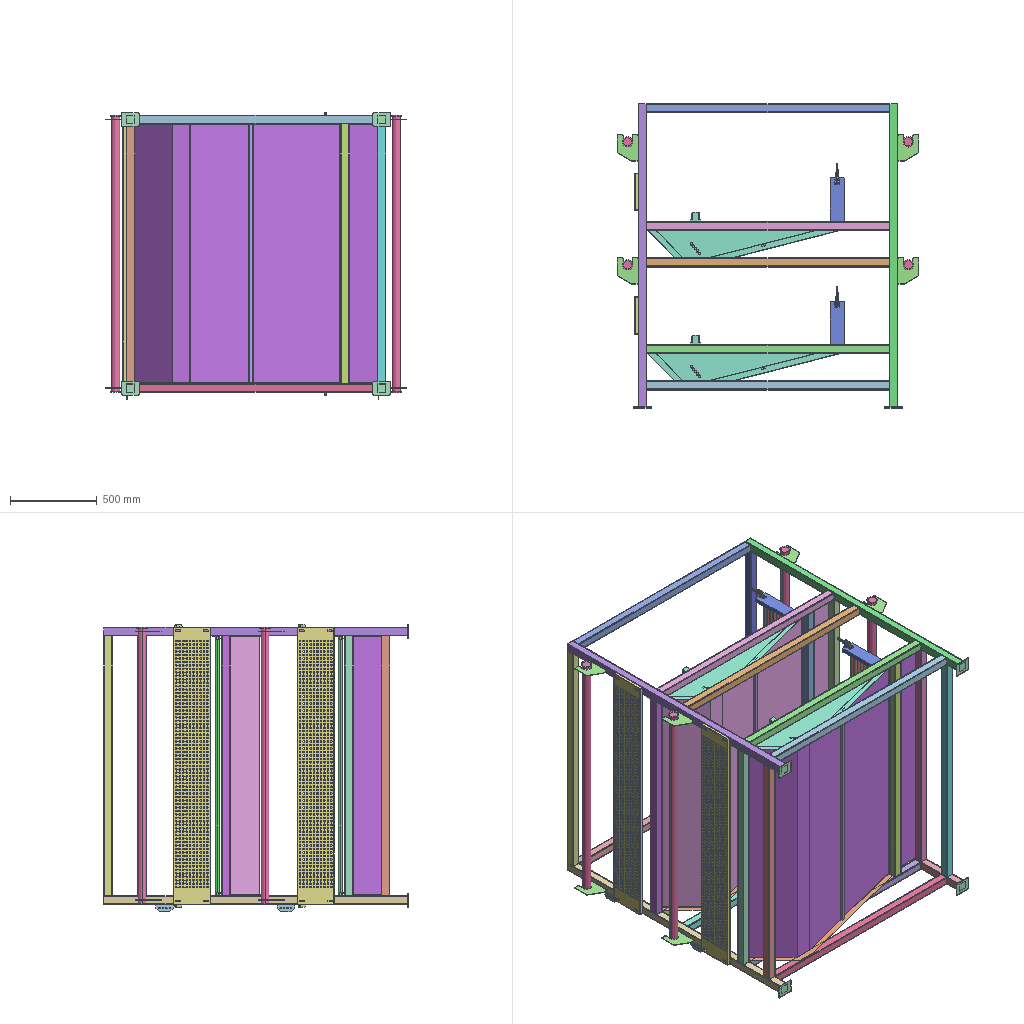Assembly | SolidWorks | 29 different items | 101 placed | box 1740 x 1755 x 1658 mm
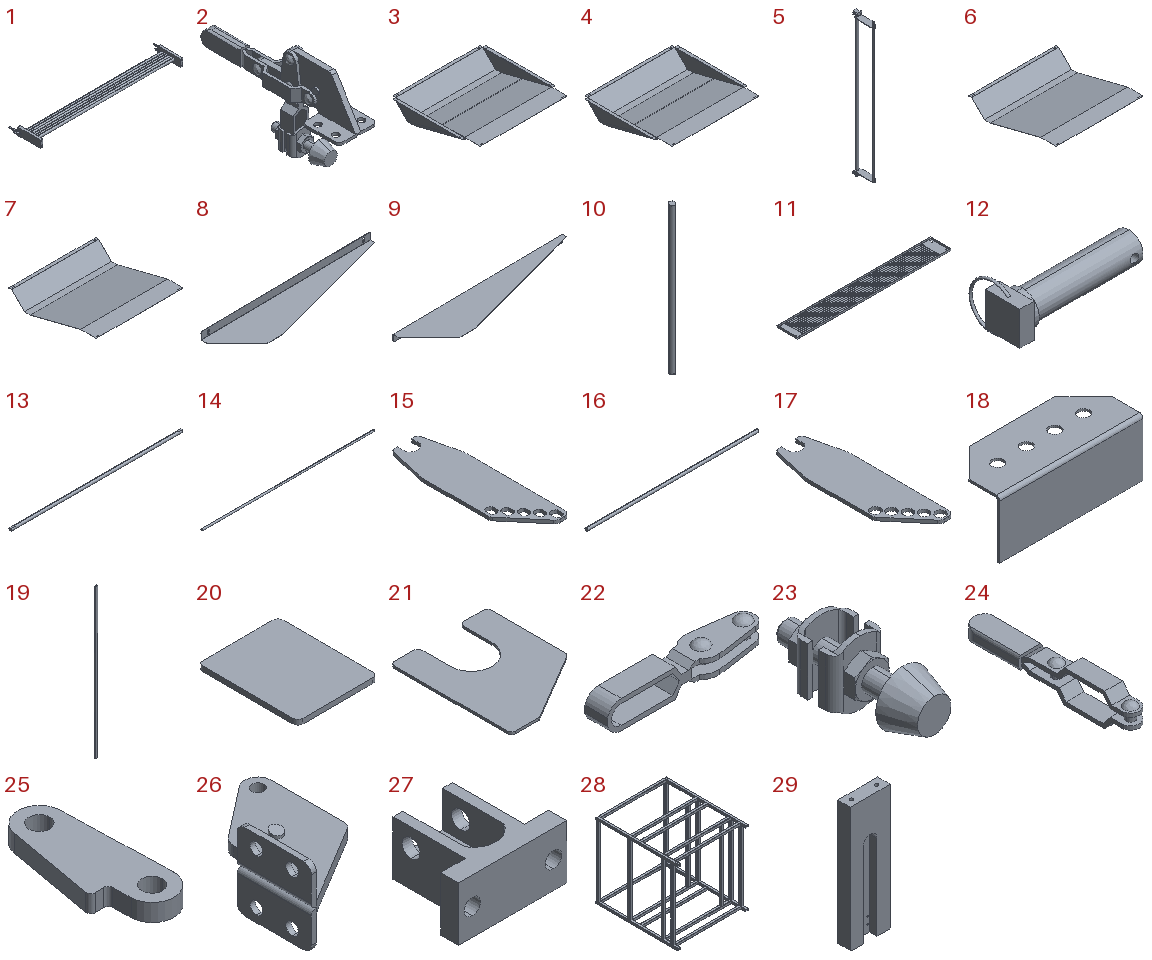Parts list (item | name | quantity | parent item | size | volume | features):
1 | (subassembly) | x2 | - | 1633 x 333.3 x 80 mm | 5408151 mm3 | features ReferencePattern 5, AEMSimFeature 1, LocalLPattern 1
2 | (subassembly) | x4 | in 1 | 30 x 119.8 x 70.25 mm | 20145 mm3 | -
3 | (subassembly) | x1 | - | 1590 x 1497 x 254.534 mm | 4476617 mm3 | -
4 | (subassembly) | x1 | - | 1590 x 1497 x 255.323 mm | 4476617 mm3 | -
5 | (subassembly) | x2 | - | 68 x 247.07 x 1556 mm | 2258393 mm3 | features ReferencePattern 4, LocalLPattern 1
6 | - | x1 | in 3 | 1490 x 1497 x 221.028 mm | 3607378 mm3 | features EdgeFlange 4, Extrusion 1, Fillet 1, FlatPattern 1, ICE 1, SheetMetal 1, SolidToSheetMetal 1
7 | - | x1 | in 4 | 1490 x 1497 x 221.028 mm | 3607378 mm3 | features EdgeFlange 4, Extrusion 1, Fillet 1, FlatPattern 1, ICE 1, SheetMetal 1, SolidToSheetMetal 1
8 | - | x2 | in 3, 4 | 1189 x 264.437 x 50 mm | 360864 mm3 | features EdgeFlange 1, Extrusion 1, Fillet 1, FlatPattern 1, ICE 1, SheetMetal 1, SolidToSheetMetal 1
9 | - | x2 | in 3, 4 | 1189 x 264.437 x 50 mm | 360864 mm3 | features EdgeFlange 1, Extrusion 1, Fillet 1, FlatPattern 1, ICE 1, SheetMetal 1, SolidToSheetMetal 1
10 | - | x4 | - | 60 x 60 x 1600 mm | 273036 mm3 | features ICE 2, Extrusion 1, Fillet 1, RefAxis 1, RevCut 1
11 | - | x2 | - | 1600 x 215 x 20 mm | 538674 mm3 | features ICE 3, EdgeFlange 1, Extrusion 1, FlatPattern 1, SheetMetal 1, SolidToSheetMetal 1
12 | - | x4 | in 5 | 45 x 19.844 x 16.686 mm | 3901 mm3 | features ICE 3, BaseBody 1, Sweep 1
13 | - | x2 | in 5 | 1530 x 25 x 25 mm | 749305 mm3 | features ICE 3, Extrusion 1, HoleWzd 1
14 | - | x10 | in 5 | 1480 x 15 x 15 mm | 261335 mm3 | features HoleWzd 2, Chamfer 1, Extrusion 1, ICE 1
15 | - | x2 | in 5 | 68 x 225 x 5 mm | 59113 mm3 | features Fillet 5, ICE 5, Extrusion 1, LPattern 1
16 | - | x12 | in 1 | 1534 x 25 x 25 mm | 753000 mm3 | features ICE 1, MirrorPattern 1, Revolution 1
17 | - | x2 | in 5 | 68 x 225 x 5 mm | 58604 mm3 | features Fillet 5, ICE 4, Extrusion 1
18 | - | x4 | - | 100 x 41.5 x 40 mm | 10986 mm3 | features Chamfer 1, EdgeFlange 1, Extrusion 1, FlatPattern 1, SheetMetal 1, SolidToSheetMetal 1
19 | - | x2 | in 3, 4 | 23 x 13 x 1490 mm | 147510 mm3 | features ExtruThin 1, WeldmentFeature 1
20 | - | x4 | - | 80 x 100 x 5 mm | 39893 mm3 | features Extrusion 1, Fillet 1
21 | - | x8 | - | 120 x 150 x 3 mm | 38115 mm3 | features Extrusion 1
22 | - | x4 | in 2 | 70.05 x 15.001 x 12.4 mm | 3515 mm3 | features BaseBody 1
23 | - | x4 | in 2 | 16 x 44.45 x 19 mm | 3867 mm3 | features BaseBody 1
24 | - | x4 | in 2 | 12.6 x 89.5 x 17.6 mm | 5262 mm3 | features BaseBody 1
25 | - | x4 | in 2 | 14.127 x 35.318 x 4 mm | 1354 mm3 | features BaseBody 1
26 | - | x4 | in 2 | 34.2 x 55.001 x 30 mm | 6148 mm3 | features BaseBody 1
27 | - | x4 | in 5 | 60 x 50 x 30 mm | 38448 mm3 | features HoleWzd 3, ICE 3, Extrusion 1
28 | - | x1 | - | 1500 x 1750 x 1600 mm | 13453168 mm3 | features 3DProfileFeature 1, WeldCornerFeat 1, WeldMemberFeat 1, WeldmentFeature 1
29 | - | x4 | in 1 | 80 x 25 x 250 mm | 424930 mm3 | features HoleWzd 5, ICE 2, MirrorPattern 2, Chamfer 1, Extrusion 1
Mates (type | each side: item.copy, entity, surface, feature):
In the top assembly
Coincident | 28.1 face plane GB 6728-1986 square hollow section 050 X 50 X 2 | 6.1 face plane Convert entities1 | 2 times
Width | 28.1 face plane GB 6728-1986 square hollow section 050 X 50 X 2 | 28.1 face plane GB 6728-1986 square hollow section 050 X 50 X 2 | 9.1 face plane Convert entities1 | 8.1 face plane Convert entities1
Coincident | 28.1 face plane GB 6728-1986 square hollow section 050 X 50 X 2 | 21.1 face plane Boss-Extrude1
Coincident | 28.1 face plane GB 6728-1986 square hollow section 050 X 50 X 2 | 21.2 face plane Boss-Extrude1
Coincident | 28.1 face plane GB 6728-1986 square hollow section 050 X 50 X 2 | 21.3 face plane Boss-Extrude1
Coincident | 28.1 face plane GB 6728-1986 square hollow section 050 X 50 X 2 | 21.4 face plane Boss-Extrude1
Width | 28.1 face plane GB 6728-1986 square hollow section 050 X 50 X 2 | 28.1 face plane GB 6728-1986 square hollow section 050 X 50 X 2 | 21.3 face plane Boss-Extrude1 | 21.3 face plane Boss-Extrude1
Width | 28.1 face plane GB 6728-1986 square hollow section 050 X 50 X 2 | 28.1 face plane GB 6728-1986 square hollow section 050 X 50 X 2 | 21.1 face plane Boss-Extrude1 | 21.1 face plane Boss-Extrude1
Coincident | 21.3 face plane Boss-Extrude1 | 21.1 face plane Boss-Extrude1
Coincident | 21.1 face plane Boss-Extrude1 | 21.2 face plane Boss-Extrude1
Coincident | 21.2 face plane Boss-Extrude1 | 21.4 face plane Boss-Extrude1
Width | 28.1 face plane GB 6728-1986 square hollow section 050 X 50 X 2 | 28.1 face plane GB 6728-1986 square hollow section 050 X 50 X 2 | 21.2 face plane Boss-Extrude1 | 21.2 face plane Boss-Extrude1
Width | 28.1 face plane GB 6728-1986 square hollow section 050 X 50 X 2 | 28.1 face plane GB 6728-1986 square hollow section 050 X 50 X 2 | 21.4 face plane Boss-Extrude1 | 21.4 face plane Boss-Extrude1
DistanceDim | 28.1 face plane GB 6728-1986 square hollow section 050 X 50 X 2 | 21.4 face plane Boss-Extrude1
Coincident | 21.4 face plane Boss-Extrude1 | 21.5 face plane Boss-Extrude1
Coincident | 28.1 face plane GB 6728-1986 square hollow section 050 X 50 X 2 | 21.5 face plane Boss-Extrude1
Coincident | 21.1 face plane Boss-Extrude1 | 21.6 face plane Boss-Extrude1
Coincident | 28.1 face plane GB 6728-1986 square hollow section 050 X 50 X 2 | 21.6 face plane Boss-Extrude1
Coincident | 21.3 face plane Boss-Extrude1 | 21.7 face plane Boss-Extrude1
Coincident | 28.1 face plane GB 6728-1986 square hollow section 050 X 50 X 2 | 21.7 face plane Boss-Extrude1
Coincident | 28.1 face plane GB 6728-1986 square hollow section 050 X 50 X 2 | 21.8 face plane Boss-Extrude1
Coincident | 21.2 face plane Boss-Extrude1 | 21.8 face plane Boss-Extrude1
Coincident | 21.5 face plane Boss-Extrude1 | 21.8 face plane Boss-Extrude1
Coincident | 21.7 face plane Boss-Extrude1 | 21.6 face plane Boss-Extrude1
Coincident | 21.7 face plane Boss-Extrude1 | 21.8 face plane Boss-Extrude1
Concentric | 21.3 edge | 10.1 face cylinder Boss-Extrude1
Width | 28.1 face plane GB 6728-1986 square hollow section 050 X 50 X 2 | 28.1 face plane GB 6728-1986 square hollow section 050 X 50 X 2 | 10.1 face plane Boss-Extrude3 | 10.1 face plane Boss-Extrude2
Concentric | 21.7 edge | 10.2 face cylinder Boss-Extrude1
Concentric | 21.2 edge | 10.3 face cylinder Boss-Extrude1
Concentric | 21.8 edge | 10.4 face cylinder Boss-Extrude1
Coincident | 18.1 face plane Edge-Flange1 | 18.2 face plane Edge-Flange1
Coincident | 18.3 face plane Edge-Flange1 | 18.4 face plane Edge-Flange1
Coincident | 28.1 face plane GB 6728-1986 square hollow section 050 X 50 X 2 | 18.2 face plane Edge-Flange1
Coincident | 28.1 face plane GB 6728-1986 square hollow section 050 X 50 X 2 | 18.3 face plane Edge-Flange1
Width | 28.1 face plane GB 6728-1986 square hollow section 050 X 50 X 2 | 28.1 face plane GB 6728-1986 square hollow section 050 X 50 X 2 | 18.1 face plane Edge-Flange1 | 18.1 face plane Convert entities1
Coincident | 28.1 face plane GB 6728-1986 square hollow section 050 X 50 X 2 | 18.1 face plane Edge-Flange1
Width | 28.1 face plane GB 6728-1986 square hollow section 050 X 50 X 2 | 28.1 face plane GB 6728-1986 square hollow section 050 X 50 X 2 | 18.4 face plane Convert entities1 | 18.4 face plane Edge-Flange1
Coincident | 28.1 face plane GB 6728-1986 square hollow section 050 X 50 X 2 | 18.4 face plane Edge-Flange1
Width | 28.1 face plane GB 6728-1986 square hollow section 050 X 50 X 2 | 28.1 face plane GB 6728-1986 square hollow section 050 X 50 X 2 | 18.3 face plane Convert entities1 | 18.3 face plane Edge-Flange1
DistanceDim | 28.1 face plane GB 6728-1986 square hollow section 050 X 50 X 2 | 18.2 face plane Edge-Flange1
DistanceDim | 18.2 face plane Edge-Flange1 | 18.3 face plane Edge-Flange1
Width | 28.1 face plane GB 6728-1986 square hollow section 050 X 50 X 2 | 28.1 face plane GB 6728-1986 square hollow section 050 X 50 X 2 | 8.2 face plane Convert entities1 | 9.2 face plane Convert entities1
Coincident | 28.1 face plane GB 6728-1986 square hollow section 050 X 50 X 2 | 7.1 face plane Convert entities1
Coincident | 6.1 face plane Convert entities1 | 7.1 face plane Convert entities1
Coincident | 10.1 face plane Boss-Extrude2 | 10.3 face plane Boss-Extrude2
Coincident | 10.3 face plane Boss-Extrude2 | 10.4 face plane Boss-Extrude2
DistanceDim | 28.1 face plane GB 6728-1986 square hollow section 050 X 50 X 2 | 11.1 face plane Edge-Flange1
DistanceDim | 21.2 face plane Boss-Extrude1 | 21.8 face plane Boss-Extrude1
Width | 28.1 face plane GB 6728-1986 square hollow section 050 X 50 X 2 | 28.1 face plane GB 6728-1986 square hollow section 050 X 50 X 2 | 20.1 face plane Boss-Extrude1 | 20.1 face plane Boss-Extrude1 | 2 times
Coincident | 28.1 face plane GB 6728-1986 square hollow section 050 X 50 X 2 | 20.1 face plane Boss-Extrude1
Width | 28.1 face plane GB 6728-1986 square hollow section 050 X 50 X 2 | 28.1 face plane GB 6728-1986 square hollow section 050 X 50 X 2 | 20.2 face plane Boss-Extrude1 | 20.2 face plane Boss-Extrude1 | 2 times
Coincident | 28.1 face plane GB 6728-1986 square hollow section 050 X 50 X 2 | 20.2 face plane Boss-Extrude1
Width | 28.1 face plane GB 6728-1986 square hollow section 050 X 50 X 2 | 28.1 face plane GB 6728-1986 square hollow section 050 X 50 X 2 | 20.3 face plane Boss-Extrude1 | 20.3 face plane Boss-Extrude1 | 2 times
Coincident | 28.1 face plane GB 6728-1986 square hollow section 050 X 50 X 2 | 20.3 face plane Boss-Extrude1
Width | 28.1 face plane GB 6728-1986 square hollow section 050 X 50 X 2 | 28.1 face plane GB 6728-1986 square hollow section 050 X 50 X 2 | 20.4 face plane Boss-Extrude1 | 20.4 face plane Boss-Extrude1 | 2 times
Coincident | 28.1 face plane GB 6728-1986 square hollow section 050 X 50 X 2 | 20.4 face plane Boss-Extrude1
DistanceDim | 11.1 face plane Edge-Flange1 | 11.2 edge
Coincident | 11.1 face plane Edge-Flange1 | 11.2 face plane Edge-Flange1
Width | 28.1 face plane GB 6728-1986 square hollow section 050 X 50 X 2 | 28.1 face plane GB 6728-1986 square hollow section 050 X 50 X 2 | 11.1 face plane Edge-Flange1 | 11.1 face plane Edge-Flange1
Coincident | 11.1 face plane Convert entities1 | 11.2 face plane Convert entities1
Coincident | 28.1 face plane GB 6728-1986 square hollow section 050 X 50 X 2 | 11.1 face plane Edge-Flange1
Coincident | 29.1 face plane Boss-Extrude1 | 29.2 face plane Boss-Extrude1 | 2 times
DistanceDim | 29.1 face plane Boss-Extrude1 | 28.1 face plane GB 6728-1986 square hollow section 050 X 50 X 2
Width | 28.1 face plane GB 6728-1986 square hollow section 050 X 50 X 2 | 28.1 face plane GB 6728-1986 square hollow section 050 X 50 X 2 | 29.3 face plane Boss-Extrude1 | 29.1 face plane Boss-Extrude1
Coincident | 28.1 face plane GB 6728-1986 square hollow section 050 X 50 X 2 | 29.2 face plane Boss-Extrude1
Coincident | assembly face | assembly face | 2 times
Width | 28.1 face plane GB 6728-1986 square hollow section 050 X 50 X 2 | 28.1 face plane GB 6728-1986 square hollow section 050 X 50 X 2 | assembly face | assembly face
Coincident | 8.1 face plane Edge-Flange1 | assembly face
In subassembly 3
Coincident | 6.2 face plane Edge-Flange1 | 9.3 face plane Convert entities1
Coincident | 6.2 face plane Edge-Flange1 | 8.3 face plane Convert entities1
Parallel | 6.2 face plane Convert entities1 | 9.3 face plane Edge-Flange1
Parallel | 6.2 face plane Convert entities1 | 8.3 face plane Edge-Flange1
Coincident | 6.2 face plane Edge-Flange3 | 19.1 face plane Extrude-Thin1
Width | 8.3 face plane Convert entities1 | 9.3 face plane Convert entities1 | 19.1 face plane Extrude-Thin1 | 19.1 face plane Extrude-Thin1
DistanceDim | 6.2 edge | 19.1 face plane Extrude-Thin1
Coincident | 8.3 face plane Convert entities1 | 19.1 face plane Extrude-Thin1
In subassembly 4
Coincident | 7.2 face plane Edge-Flange1 | 8.4 face plane Convert entities1
Coincident | 7.2 face plane Edge-Flange1 | 9.3 face plane Convert entities1
Coincident | 8.4 face plane Convert entities1 | 9.3 face plane Convert entities1
Parallel | 7.2 face plane Convert entities1 | 8.4 face plane Edge-Flange1
Parallel | 7.2 face plane Convert entities1 | 9.3 face plane Edge-Flange1
Coincident | 7.2 face plane Edge-Flange3 | 19.1 face plane Extrude-Thin1
Coincident | 9.3 face plane Convert entities1 | 19.1 face plane Extrude-Thin1
DistanceDim | 7.2 edge | 19.1 edge
In subassembly 1
Concentric | 16.1 face cylinder Revolve1 | 29.4 face cylinder Cut-Extrude1
Coincident | 29.5 face plane Boss-Extrude1 | 29.4 face plane Boss-Extrude1
Concentric | 16.1 face cylinder Revolve1 | 29.5 face cylinder Cut-Extrude1
DistanceDim | 29.5 face plane Boss-Extrude1 | 29.4 face plane Boss-Extrude1
Parallel | 16.1 plane | 29.5 face plane Boss-Extrude1
Width | 29.5 face plane Boss-Extrude1 | 29.4 face plane Boss-Extrude1 | 16.1 face plane Mirror1 | 16.1 face plane Revolve1
Coincident | 29.4 face plane Boss-Extrude1 | 26.1 face plane Import1
Width | 26.1 face plane Import1 | 26.1 face plane Import1 | 29.4 face plane Boss-Extrude1 | 29.4 face plane Boss-Extrude1
DistanceDim | 26.1 face plane Import1 | 29.4 face plane Boss-Extrude1
Coincident | 29.5 face plane Boss-Extrude1 | 26.2 face plane Import1
Coincident | 26.1 face plane Import1 | 26.2 face plane Import1 | 2 times
In subassembly 5
Concentric | 13.1 face cylinder Boss-Extrude1 | 17.1 face cylinder Cut-Extrude3
Concentric | 13.1 face cylinder Boss-Extrude1 | 15.1 face cylinder Cut-Extrude3
DistanceDim | 15.1 face plane Boss-Extrude1 | 17.1 face plane Boss-Extrude1
Concentric | 14.1 face cylinder Boss-Extrude1 | 15.1 face cylinder Cut-Extrude1
Parallel | 14.1 face plane Cut-Extrude1 | 15.1 face plane LPattern1
Parallel | 13.1 face plane Cut-Extrude1 | 15.1 face plane Cut-Extrude3
Concentric | 12.1 face cylinder Import1 | 27.1 face cylinder Ø10.0 (10) Diameter Hole1
Coincident | 12.1 face plane Import1 | 27.1 face plane Cut-Extrude2
Concentric | 12.2 face cylinder Import1 | 27.2 face cylinder Ø10.0 (10) Diameter Hole2
Coincident | 12.2 face plane Import1 | 27.2 face plane Cut-Extrude1
DistanceDim | 13.1 face cylinder Boss-Extrude1 | 27.1 face cylinder Cut-Extrude3
Coincident | 27.1 face plane Boss-Extrude1 | 27.2 face plane Boss-Extrude1
Parallel | 27.1 face plane Cut-Extrude2 | 27.2 face plane Cut-Extrude1
Width | 27.1 face plane Cut-Extrude3 | 27.1 face plane Cut-Extrude3 | 13.1 face plane Cut-Extrude1 | 13.1 face plane Cut-Extrude2
DistanceDim | 27.1 face plane Cut-Extrude3 | 13.1 face plane Boss-Extrude1
DistanceDim | 13.1 face plane Boss-Extrude1 | 27.2 face plane Cut-Extrude3
Width | 13.1 face plane Cut-Extrude2 | 13.1 face plane Cut-Extrude1 | 27.2 face plane Cut-Extrude3 | 27.2 face plane Cut-Extrude3
Width | 27.2 face plane Boss-Extrude1 | 27.1 face plane Boss-Extrude1 | 15.1 face plane Boss-Extrude1 | 17.1 face plane Boss-Extrude1
Coincident | 13.1 face plane Cut-Extrude2 | 17.1 face plane Cut-Extrude3
Coincident | 14.1 face plane Cut-Extrude1 | 15.1 face plane Boss-Extrude1